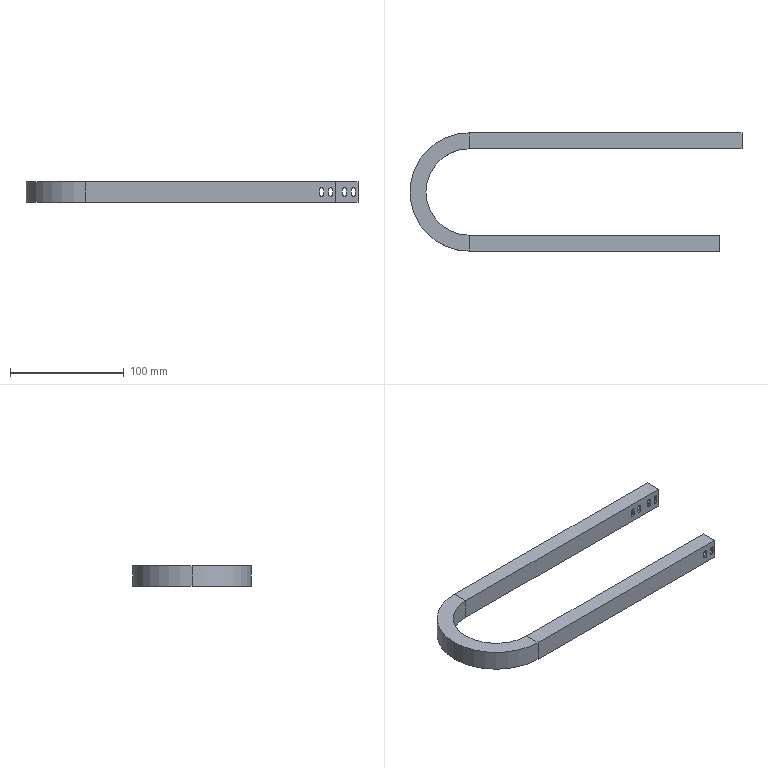Part | NX | features BREP 1 | 1 solid | 78 faces | box 292 x 104 x 18 mm | volume 90842 mm3 | plane 46 | cylinder 32 | commonest cylinder face diameters 3.5 x24 76 x2 80 x2 100 x2 104 x2